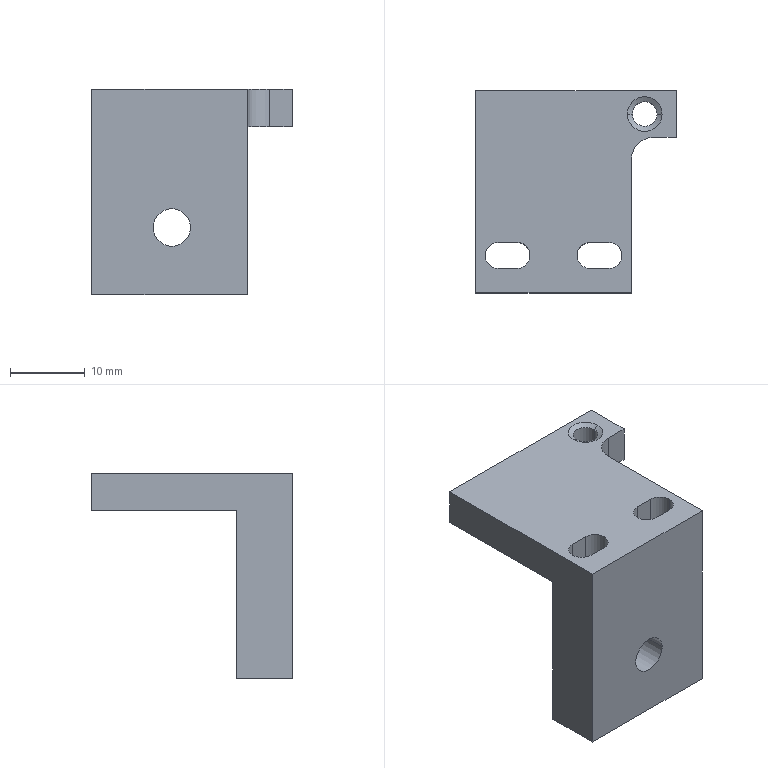Part | NX | 1 solid | 27 faces | box 26.8 x 27 x 27.5 mm | volume 5312 mm3 | plane 14 | cylinder 11 | cone 2 | commonest cylinder face diameters 3.5 x6 3.3 x2 5 x2 6 x1
STEP:
#1=CARTESIAN_POINT('',(6.,-2.5,-13.75));
#2=VERTEX_POINT('',#1);
#3=CARTESIAN_POINT('',(6.,-10.,-13.75));
#4=VERTEX_POINT('',#3);
#5=CARTESIAN_POINT('',(6.,0.,-13.75));
#6=DIRECTION('',(0.,-1.,0.));
#7=VECTOR('',#6,1000.);
#8=LINE('',#5,#7);
#9=EDGE_CURVE('',#2,#4,#8,.T.);
#10=ORIENTED_EDGE('',*,*,#9,.F.);
#11=CARTESIAN_POINT('',(6.,-2.5,8.75));
#12=VERTEX_POINT('',#11);
#13=CARTESIAN_POINT('',(6.,-2.5,0.));
#14=DIRECTION('',(0.,0.,1.));
#15=VECTOR('',#14,1000.);
#16=LINE('',#13,#15);
#17=EDGE_CURVE('',#2,#12,#16,.T.);
#18=ORIENTED_EDGE('',*,*,#17,.T.);
#19=CARTESIAN_POINT('',(6.,7.8,8.75));
#20=VERTEX_POINT('',#19);
#21=CARTESIAN_POINT('',(6.,0.,8.75));
#22=DIRECTION('',(0.,1.,0.));
#23=VECTOR('',#22,1000.);
#24=LINE('',#21,#23);
#25=EDGE_CURVE('',#12,#20,#24,.T.);
#26=ORIENTED_EDGE('',*,*,#25,.T.);
#27=CARTESIAN_POINT('',(6.,7.8,13.75));
#28=VERTEX_POINT('',#27);
#29=CARTESIAN_POINT('',(6.,7.8,0.));
#30=DIRECTION('',(0.,0.,1.));
#31=VECTOR('',#30,1000.);
#32=LINE('',#29,#31);
#33=EDGE_CURVE('',#20,#28,#32,.T.);
#34=ORIENTED_EDGE('',*,*,#33,.T.);
#35=CARTESIAN_POINT('',(6.,-10.,13.75));
#36=VERTEX_POINT('',#35);
#37=CARTESIAN_POINT('',(6.,0.,13.75));
#38=DIRECTION('',(0.,1.,0.));
#39=VECTOR('',#38,1000.);
#40=LINE('',#37,#39);
#41=EDGE_CURVE('',#36,#28,#40,.T.);
#42=ORIENTED_EDGE('',*,*,#41,.F.);
#43=CARTESIAN_POINT('',(6.,-10.,0.));
#44=DIRECTION('',(0.,0.,1.));
#45=VECTOR('',#44,1000.);
#46=LINE('',#43,#45);
#47=EDGE_CURVE('',#4,#36,#46,.T.);
#48=ORIENTED_EDGE('',*,*,#47,.F.);
#49=EDGE_LOOP('',(#10,#18,#26,#34,#42,#48));
#50=FACE_BOUND('',#49,.T.);
#51=CARTESIAN_POINT('',(6.,0.,0.));
#52=DIRECTION('',(-1.,0.,0.));
#53=DIRECTION('',(0.,0.,1.));
#54=AXIS2_PLACEMENT_3D('',#51,#52,#53);
#55=PLANE('',#54);
#56=ADVANCED_FACE('',(#50),#55,.F.);
#57=CARTESIAN_POINT('',(-14.8,-2.5,8.75));
#58=VERTEX_POINT('',#57);
#59=CARTESIAN_POINT('',(0.,-2.5,8.75));
#60=DIRECTION('',(-1.,0.,0.));
#61=VECTOR('',#60,1000.);
#62=LINE('',#59,#61);
#63=EDGE_CURVE('',#12,#58,#62,.T.);
#64=ORIENTED_EDGE('',*,*,#63,.F.);
#65=ORIENTED_EDGE('',*,*,#17,.F.);
#66=CARTESIAN_POINT('',(-14.8,-2.5,-13.75));
#67=VERTEX_POINT('',#66);
#68=CARTESIAN_POINT('',(0.,-2.5,-13.75));
#69=DIRECTION('',(1.,0.,0.));
#70=VECTOR('',#69,1000.);
#71=LINE('',#68,#70);
#72=EDGE_CURVE('',#67,#2,#71,.T.);
#73=ORIENTED_EDGE('',*,*,#72,.F.);
#74=CARTESIAN_POINT('',(-14.8,-2.5,0.));
#75=DIRECTION('',(0.,0.,-1.));
#76=VECTOR('',#75,1000.);
#77=LINE('',#74,#76);
#78=EDGE_CURVE('',#58,#67,#77,.T.);
#79=ORIENTED_EDGE('',*,*,#78,.F.);
#80=EDGE_LOOP('',(#64,#65,#73,#79));
#81=FACE_BOUND('',#80,.T.);
#82=CARTESIAN_POINT('',(-6.6,-2.5,-4.75));
#83=VERTEX_POINT('',#82);
#84=CARTESIAN_POINT('',(-1.6,-2.5,-4.75));
#85=VERTEX_POINT('',#84);
#86=CARTESIAN_POINT('',(-4.1,-2.5,-4.75));
#87=DIRECTION('',(0.,1.,0.));
#88=DIRECTION('',(-1.,0.,0.));
#89=AXIS2_PLACEMENT_3D('',#86,#87,#88);
#90=CIRCLE('',#89,2.5);
#91=EDGE_CURVE('',#83,#85,#90,.T.);
#92=ORIENTED_EDGE('',*,*,#91,.F.);
#93=CARTESIAN_POINT('',(-4.1,-2.5,-4.75));
#94=DIRECTION('',(0.,1.,0.));
#95=DIRECTION('',(-1.,0.,0.));
#96=AXIS2_PLACEMENT_3D('',#93,#94,#95);
#97=CIRCLE('',#96,2.5);
#98=EDGE_CURVE('',#85,#83,#97,.T.);
#99=ORIENTED_EDGE('',*,*,#98,.F.);
#100=EDGE_LOOP('',(#92,#99));
#101=FACE_BOUND('',#100,.T.);
#102=CARTESIAN_POINT('',(0.,-2.5,8.75));
#103=DIRECTION('',(0.,-1.,0.));
#104=DIRECTION('',(0.,0.,-1.));
#105=AXIS2_PLACEMENT_3D('',#102,#103,#104);
#106=PLANE('',#105);
#107=ADVANCED_FACE('',(#81,#101),#106,.F.);
#108=CARTESIAN_POINT('',(9.,10.8,8.75));
#109=VERTEX_POINT('',#108);
#110=CARTESIAN_POINT('',(9.,10.8,13.75));
#111=VERTEX_POINT('',#110);
#112=CARTESIAN_POINT('',(9.,10.8,0.));
#113=DIRECTION('',(0.,0.,1.));
#114=VECTOR('',#113,1000.);
#115=LINE('',#112,#114);
#116=EDGE_CURVE('',#109,#111,#115,.T.);
#117=ORIENTED_EDGE('',*,*,#116,.F.);
#118=CARTESIAN_POINT('',(12.,10.8,8.75));
#119=VERTEX_POINT('',#118);
#120=CARTESIAN_POINT('',(0.,10.8,8.75));
#121=DIRECTION('',(-1.,0.,0.));
#122=VECTOR('',#121,1000.);
#123=LINE('',#120,#122);
#124=EDGE_CURVE('',#119,#109,#123,.T.);
#125=ORIENTED_EDGE('',*,*,#124,.F.);
#126=CARTESIAN_POINT('',(12.,10.8,13.75));
#127=VERTEX_POINT('',#126);
#128=CARTESIAN_POINT('',(12.,10.8,13.75));
#129=DIRECTION('',(0.,0.,-1.));
#130=VECTOR('',#129,1000.);
#131=LINE('',#128,#130);
#132=EDGE_CURVE('',#127,#119,#131,.T.);
#133=ORIENTED_EDGE('',*,*,#132,.F.);
#134=CARTESIAN_POINT('',(0.,10.8,13.75));
#135=DIRECTION('',(-1.,0.,0.));
#136=VECTOR('',#135,1000.);
#137=LINE('',#134,#136);
#138=EDGE_CURVE('',#127,#111,#137,.T.);
#139=ORIENTED_EDGE('',*,*,#138,.T.);
#140=EDGE_LOOP('',(#117,#125,#133,#139));
#141=FACE_BOUND('',#140,.T.);
#142=CARTESIAN_POINT('',(6.,10.8,13.75));
#143=DIRECTION('',(0.,-1.,0.));
#144=DIRECTION('',(0.,0.,-1.));
#145=AXIS2_PLACEMENT_3D('',#142,#143,#144);
#146=PLANE('',#145);
#147=ADVANCED_FACE('',(#141),#146,.T.);
#148=ORIENTED_EDGE('',*,*,#78,.T.);
#149=CARTESIAN_POINT('',(-14.8,-10.,-13.75));
#150=VERTEX_POINT('',#149);
#151=CARTESIAN_POINT('',(-14.8,0.,-13.75));
#152=DIRECTION('',(0.,-1.,0.));
#153=VECTOR('',#152,1000.);
#154=LINE('',#151,#153);
#155=EDGE_CURVE('',#67,#150,#154,.T.);
#156=ORIENTED_EDGE('',*,*,#155,.T.);
#157=CARTESIAN_POINT('',(-14.8,-10.,13.75));
#158=VERTEX_POINT('',#157);
#159=CARTESIAN_POINT('',(-14.8,-10.,0.));
#160=DIRECTION('',(0.,0.,-1.));
#161=VECTOR('',#160,1000.);
#162=LINE('',#159,#161);
#163=EDGE_CURVE('',#158,#150,#162,.T.);
#164=ORIENTED_EDGE('',*,*,#163,.F.);
#165=CARTESIAN_POINT('',(-14.8,17.,13.75));
#166=VERTEX_POINT('',#165);
#167=CARTESIAN_POINT('',(-14.8,0.,13.75));
#168=DIRECTION('',(0.,1.,0.));
#169=VECTOR('',#168,1000.);
#170=LINE('',#167,#169);
#171=EDGE_CURVE('',#158,#166,#170,.T.);
#172=ORIENTED_EDGE('',*,*,#171,.T.);
#173=CARTESIAN_POINT('',(-14.8,17.,8.75));
#174=VERTEX_POINT('',#173);
#175=CARTESIAN_POINT('',(-14.8,17.,0.));
#176=DIRECTION('',(0.,0.,1.));
#177=VECTOR('',#176,1000.);
#178=LINE('',#175,#177);
#179=EDGE_CURVE('',#174,#166,#178,.T.);
#180=ORIENTED_EDGE('',*,*,#179,.F.);
#181=CARTESIAN_POINT('',(-14.8,0.,8.75));
#182=DIRECTION('',(0.,-1.,0.));
#183=VECTOR('',#182,1000.);
#184=LINE('',#181,#183);
#185=EDGE_CURVE('',#174,#58,#184,.T.);
#186=ORIENTED_EDGE('',*,*,#185,.T.);
#187=EDGE_LOOP('',(#148,#156,#164,#172,#180,#186));
#188=FACE_BOUND('',#187,.T.);
#189=CARTESIAN_POINT('',(-14.8,0.,0.));
#190=DIRECTION('',(-1.,0.,0.));
#191=DIRECTION('',(0.,0.,1.));
#192=AXIS2_PLACEMENT_3D('',#189,#190,#191);
#193=PLANE('',#192);
#194=ADVANCED_FACE('',(#188),#193,.T.);
#195=CARTESIAN_POINT('',(12.,17.,13.75));
#196=VERTEX_POINT('',#195);
#197=CARTESIAN_POINT('',(12.,0.,13.75));
#198=DIRECTION('',(0.,-1.,0.));
#199=VECTOR('',#198,1000.);
#200=LINE('',#197,#199);
#201=EDGE_CURVE('',#196,#127,#200,.T.);
#202=ORIENTED_EDGE('',*,*,#201,.T.);
#203=ORIENTED_EDGE('',*,*,#132,.T.);
#204=CARTESIAN_POINT('',(12.,17.,8.75));
#205=VERTEX_POINT('',#204);
#206=CARTESIAN_POINT('',(12.,0.,8.75));
#207=DIRECTION('',(0.,-1.,0.));
#208=VECTOR('',#207,1000.);
#209=LINE('',#206,#208);
#210=EDGE_CURVE('',#205,#119,#209,.T.);
#211=ORIENTED_EDGE('',*,*,#210,.F.);
#212=CARTESIAN_POINT('',(12.,17.,0.));
#213=DIRECTION('',(0.,0.,1.));
#214=VECTOR('',#213,1000.);
#215=LINE('',#212,#214);
#216=EDGE_CURVE('',#205,#196,#215,.T.);
#217=ORIENTED_EDGE('',*,*,#216,.T.);
#218=EDGE_LOOP('',(#202,#203,#211,#217));
#219=FACE_BOUND('',#218,.T.);
#220=CARTESIAN_POINT('',(12.,10.8,13.75));
#221=DIRECTION('',(1.,0.,0.));
#222=DIRECTION('',(0.,1.,0.));
#223=AXIS2_PLACEMENT_3D('',#220,#221,#222);
#224=PLANE('',#223);
#225=ADVANCED_FACE('',(#219),#224,.T.);
#226=CARTESIAN_POINT('',(0.,17.,13.75));
#227=DIRECTION('',(1.,0.,0.));
#228=VECTOR('',#227,1000.);
#229=LINE('',#226,#228);
#230=EDGE_CURVE('',#166,#196,#229,.T.);
#231=ORIENTED_EDGE('',*,*,#230,.T.);
#232=ORIENTED_EDGE('',*,*,#216,.F.);
#233=CARTESIAN_POINT('',(0.,17.,8.75));
#234=DIRECTION('',(1.,0.,0.));
#235=VECTOR('',#234,1000.);
#236=LINE('',#233,#235);
#237=EDGE_CURVE('',#174,#205,#236,.T.);
#238=ORIENTED_EDGE('',*,*,#237,.F.);
#239=ORIENTED_EDGE('',*,*,#179,.T.);
#240=EDGE_LOOP('',(#231,#232,#238,#239));
#241=FACE_BOUND('',#240,.T.);
#242=CARTESIAN_POINT('',(12.,17.,13.75));
#243=DIRECTION('',(0.,1.,0.));
#244=DIRECTION('',(1.,0.,0.));
#245=AXIS2_PLACEMENT_3D('',#242,#243,#244);
#246=PLANE('',#245);
#247=ADVANCED_FACE('',(#241),#246,.T.);
#248=CARTESIAN_POINT('',(0.,-10.,13.75));
#249=DIRECTION('',(-1.,0.,0.));
#250=VECTOR('',#249,1000.);
#251=LINE('',#248,#250);
#252=EDGE_CURVE('',#36,#158,#251,.T.);
#253=ORIENTED_EDGE('',*,*,#252,.T.);
#254=ORIENTED_EDGE('',*,*,#163,.T.);
#255=CARTESIAN_POINT('',(0.,-10.,-13.75));
#256=DIRECTION('',(1.,0.,0.));
#257=VECTOR('',#256,1000.);
#258=LINE('',#255,#257);
#259=EDGE_CURVE('',#150,#4,#258,.T.);
#260=ORIENTED_EDGE('',*,*,#259,.T.);
#261=ORIENTED_EDGE('',*,*,#47,.T.);
#262=EDGE_LOOP('',(#253,#254,#260,#261));
#263=FACE_BOUND('',#262,.T.);
#264=CARTESIAN_POINT('',(-6.6,-10.,-4.75));
#265=VERTEX_POINT('',#264);
#266=CARTESIAN_POINT('',(-1.6,-10.,-4.75));
#267=VERTEX_POINT('',#266);
#268=CARTESIAN_POINT('',(-4.1,-10.,-4.75));
#269=DIRECTION('',(0.,1.,0.));
#270=DIRECTION('',(-1.,0.,0.));
#271=AXIS2_PLACEMENT_3D('',#268,#269,#270);
#272=CIRCLE('',#271,2.5);
#273=EDGE_CURVE('',#265,#267,#272,.T.);
#274=ORIENTED_EDGE('',*,*,#273,.T.);
#275=CARTESIAN_POINT('',(-4.1,-10.,-4.75));
#276=DIRECTION('',(0.,1.,0.));
#277=DIRECTION('',(-1.,0.,0.));
#278=AXIS2_PLACEMENT_3D('',#275,#276,#277);
#279=CIRCLE('',#278,2.5);
#280=EDGE_CURVE('',#267,#265,#279,.T.);
#281=ORIENTED_EDGE('',*,*,#280,.T.);
#282=EDGE_LOOP('',(#274,#281));
#283=FACE_BOUND('',#282,.T.);
#284=CARTESIAN_POINT('',(0.,-10.,-13.75));
#285=DIRECTION('',(0.,-1.,0.));
#286=DIRECTION('',(0.,0.,-1.));
#287=AXIS2_PLACEMENT_3D('',#284,#285,#286);
#288=PLANE('',#287);
#289=ADVANCED_FACE('',(#263,#283),#288,.T.);
#290=ORIENTED_EDGE('',*,*,#9,.T.);
#291=ORIENTED_EDGE('',*,*,#259,.F.);
#292=ORIENTED_EDGE('',*,*,#155,.F.);
#293=ORIENTED_EDGE('',*,*,#72,.T.);
#294=EDGE_LOOP('',(#290,#291,#292,#293));
#295=FACE_BOUND('',#294,.T.);
#296=CARTESIAN_POINT('',(-11.8,-6.75,-13.75));
#297=VERTEX_POINT('',#296);
#298=CARTESIAN_POINT('',(-13.55,-5.,-13.75));
#299=VERTEX_POINT('',#298);
#300=CARTESIAN_POINT('',(-11.8,-5.,-13.75));
#301=DIRECTION('',(0.,0.,-1.));
#302=DIRECTION('',(-1.,0.,0.));
#303=AXIS2_PLACEMENT_3D('',#300,#301,#302);
#304=CIRCLE('',#303,1.75);
#305=EDGE_CURVE('',#297,#299,#304,.T.);
#306=ORIENTED_EDGE('',*,*,#305,.F.);
#307=CARTESIAN_POINT('',(-9.3,-6.75,-13.75));
#308=VERTEX_POINT('',#307);
#309=CARTESIAN_POINT('',(0.,-6.75,-13.75));
#310=DIRECTION('',(1.,0.,0.));
#311=VECTOR('',#310,1000.);
#312=LINE('',#309,#311);
#313=EDGE_CURVE('',#297,#308,#312,.T.);
#314=ORIENTED_EDGE('',*,*,#313,.T.);
#315=CARTESIAN_POINT('',(-9.3,-3.25,-13.75));
#316=VERTEX_POINT('',#315);
#317=CARTESIAN_POINT('',(-9.3,-5.,-13.75));
#318=DIRECTION('',(0.,0.,-1.));
#319=DIRECTION('',(-1.,0.,0.));
#320=AXIS2_PLACEMENT_3D('',#317,#318,#319);
#321=CIRCLE('',#320,1.75);
#322=EDGE_CURVE('',#316,#308,#321,.T.);
#323=ORIENTED_EDGE('',*,*,#322,.F.);
#324=CARTESIAN_POINT('',(-11.8,-3.25,-13.75));
#325=VERTEX_POINT('',#324);
#326=CARTESIAN_POINT('',(0.,-3.25,-13.75));
#327=DIRECTION('',(1.,0.,0.));
#328=VECTOR('',#327,1000.);
#329=LINE('',#326,#328);
#330=EDGE_CURVE('',#325,#316,#329,.T.);
#331=ORIENTED_EDGE('',*,*,#330,.F.);
#332=CARTESIAN_POINT('',(-11.8,-5.,-13.75));
#333=DIRECTION('',(0.,0.,-1.));
#334=DIRECTION('',(-1.,0.,0.));
#335=AXIS2_PLACEMENT_3D('',#332,#333,#334);
#336=CIRCLE('',#335,1.75);
#337=EDGE_CURVE('',#299,#325,#336,.T.);
#338=ORIENTED_EDGE('',*,*,#337,.F.);
#339=EDGE_LOOP('',(#306,#314,#323,#331,#338));
#340=FACE_BOUND('',#339,.T.);
#341=CARTESIAN_POINT('',(3.,-6.75,-13.75));
#342=VERTEX_POINT('',#341);
#343=CARTESIAN_POINT('',(4.75,-5.,-13.75));
#344=VERTEX_POINT('',#343);
#345=CARTESIAN_POINT('',(3.,-5.,-13.75));
#346=DIRECTION('',(0.,0.,1.));
#347=DIRECTION('',(1.,0.,0.));
#348=AXIS2_PLACEMENT_3D('',#345,#346,#347);
#349=CIRCLE('',#348,1.75);
#350=EDGE_CURVE('',#342,#344,#349,.T.);
#351=ORIENTED_EDGE('',*,*,#350,.T.);
#352=CARTESIAN_POINT('',(3.,-3.25,-13.75));
#353=VERTEX_POINT('',#352);
#354=CARTESIAN_POINT('',(3.,-5.,-13.75));
#355=DIRECTION('',(0.,0.,1.));
#356=DIRECTION('',(1.,0.,0.));
#357=AXIS2_PLACEMENT_3D('',#354,#355,#356);
#358=CIRCLE('',#357,1.75);
#359=EDGE_CURVE('',#344,#353,#358,.T.);
#360=ORIENTED_EDGE('',*,*,#359,.T.);
#361=CARTESIAN_POINT('',(0.5,-3.25,-13.75));
#362=VERTEX_POINT('',#361);
#363=CARTESIAN_POINT('',(0.,-3.25,-13.75));
#364=DIRECTION('',(1.,0.,0.));
#365=VECTOR('',#364,1000.);
#366=LINE('',#363,#365);
#367=EDGE_CURVE('',#362,#353,#366,.T.);
#368=ORIENTED_EDGE('',*,*,#367,.F.);
#369=CARTESIAN_POINT('',(0.5,-6.75,-13.75));
#370=VERTEX_POINT('',#369);
#371=CARTESIAN_POINT('',(0.5,-5.,-13.75));
#372=DIRECTION('',(0.,0.,1.));
#373=DIRECTION('',(1.,0.,0.));
#374=AXIS2_PLACEMENT_3D('',#371,#372,#373);
#375=CIRCLE('',#374,1.75);
#376=EDGE_CURVE('',#362,#370,#375,.T.);
#377=ORIENTED_EDGE('',*,*,#376,.T.);
#378=CARTESIAN_POINT('',(0.,-6.75,-13.75));
#379=DIRECTION('',(-1.,0.,0.));
#380=VECTOR('',#379,1000.);
#381=LINE('',#378,#380);
#382=EDGE_CURVE('',#342,#370,#381,.T.);
#383=ORIENTED_EDGE('',*,*,#382,.F.);
#384=EDGE_LOOP('',(#351,#360,#368,#377,#383));
#385=FACE_BOUND('',#384,.T.);
#386=CARTESIAN_POINT('',(0.,17.,-13.75));
#387=DIRECTION('',(0.,0.,-1.));
#388=DIRECTION('',(0.,-1.,0.));
#389=AXIS2_PLACEMENT_3D('',#386,#387,#388);
#390=PLANE('',#389);
#391=ADVANCED_FACE('',(#295,#340,#385),#390,.T.);
#392=ORIENTED_EDGE('',*,*,#230,.F.);
#393=ORIENTED_EDGE('',*,*,#171,.F.);
#394=ORIENTED_EDGE('',*,*,#252,.F.);
#395=ORIENTED_EDGE('',*,*,#41,.T.);
#396=CARTESIAN_POINT('',(9.,7.8,13.75));
#397=DIRECTION('',(0.,0.,1.));
#398=DIRECTION('',(1.,0.,0.));
#399=AXIS2_PLACEMENT_3D('',#396,#397,#398);
#400=CIRCLE('',#399,3.);
#401=EDGE_CURVE('',#111,#28,#400,.T.);
#402=ORIENTED_EDGE('',*,*,#401,.F.);
#403=ORIENTED_EDGE('',*,*,#138,.F.);
#404=ORIENTED_EDGE('',*,*,#201,.F.);
#405=EDGE_LOOP('',(#392,#393,#394,#395,#402,#403,#404));
#406=FACE_BOUND('',#405,.T.);
#407=CARTESIAN_POINT('',(-9.3,-3.25,13.75));
#408=VERTEX_POINT('',#407);
#409=CARTESIAN_POINT('',(-9.3,-6.75,13.75));
#410=VERTEX_POINT('',#409);
#411=CARTESIAN_POINT('',(-9.3,-5.,13.75));
#412=DIRECTION('',(0.,0.,-1.));
#413=DIRECTION('',(-1.,0.,0.));
#414=AXIS2_PLACEMENT_3D('',#411,#412,#413);
#415=CIRCLE('',#414,1.75);
#416=EDGE_CURVE('',#408,#410,#415,.T.);
#417=ORIENTED_EDGE('',*,*,#416,.T.);
#418=CARTESIAN_POINT('',(-11.8,-6.75,13.75));
#419=VERTEX_POINT('',#418);
#420=CARTESIAN_POINT('',(0.,-6.75,13.75));
#421=DIRECTION('',(-1.,0.,0.));
#422=VECTOR('',#421,1000.);
#423=LINE('',#420,#422);
#424=EDGE_CURVE('',#410,#419,#423,.T.);
#425=ORIENTED_EDGE('',*,*,#424,.T.);
#426=CARTESIAN_POINT('',(-13.55,-5.,13.75));
#427=VERTEX_POINT('',#426);
#428=CARTESIAN_POINT('',(-11.8,-5.,13.75));
#429=DIRECTION('',(0.,0.,-1.));
#430=DIRECTION('',(-1.,0.,0.));
#431=AXIS2_PLACEMENT_3D('',#428,#429,#430);
#432=CIRCLE('',#431,1.75);
#433=EDGE_CURVE('',#419,#427,#432,.T.);
#434=ORIENTED_EDGE('',*,*,#433,.T.);
#435=CARTESIAN_POINT('',(-11.8,-3.25,13.75));
#436=VERTEX_POINT('',#435);
#437=CARTESIAN_POINT('',(-11.8,-5.,13.75));
#438=DIRECTION('',(0.,0.,-1.));
#439=DIRECTION('',(-1.,0.,0.));
#440=AXIS2_PLACEMENT_3D('',#437,#438,#439);
#441=CIRCLE('',#440,1.75);
#442=EDGE_CURVE('',#427,#436,#441,.T.);
#443=ORIENTED_EDGE('',*,*,#442,.T.);
#444=CARTESIAN_POINT('',(0.,-3.25,13.75));
#445=DIRECTION('',(1.,0.,0.));
#446=VECTOR('',#445,1000.);
#447=LINE('',#444,#446);
#448=EDGE_CURVE('',#436,#408,#447,.T.);
#449=ORIENTED_EDGE('',*,*,#448,.T.);
#450=EDGE_LOOP('',(#417,#425,#434,#443,#449));
#451=FACE_BOUND('',#450,.T.);
#452=CARTESIAN_POINT('',(10.115,13.9,13.75));
#453=VERTEX_POINT('',#452);
#454=CARTESIAN_POINT('',(5.485,13.9,13.75));
#455=VERTEX_POINT('',#454);
#456=CARTESIAN_POINT('',(7.8,13.9,13.75));
#457=DIRECTION('',(0.,0.,1.));
#458=DIRECTION('',(1.,0.,0.));
#459=AXIS2_PLACEMENT_3D('',#456,#457,#458);
#460=CIRCLE('',#459,2.315);
#461=EDGE_CURVE('',#453,#455,#460,.T.);
#462=ORIENTED_EDGE('',*,*,#461,.F.);
#463=CARTESIAN_POINT('',(7.8,13.9,13.75));
#464=DIRECTION('',(0.,0.,1.));
#465=DIRECTION('',(1.,0.,0.));
#466=AXIS2_PLACEMENT_3D('',#463,#464,#465);
#467=CIRCLE('',#466,2.315);
#468=EDGE_CURVE('',#455,#453,#467,.T.);
#469=ORIENTED_EDGE('',*,*,#468,.F.);
#470=EDGE_LOOP('',(#462,#469));
#471=FACE_BOUND('',#470,.T.);
#472=CARTESIAN_POINT('',(3.,-6.75,13.75));
#473=VERTEX_POINT('',#472);
#474=CARTESIAN_POINT('',(4.75,-5.,13.75));
#475=VERTEX_POINT('',#474);
#476=CARTESIAN_POINT('',(3.,-5.,13.75));
#477=DIRECTION('',(0.,0.,1.));
#478=DIRECTION('',(1.,0.,0.));
#479=AXIS2_PLACEMENT_3D('',#476,#477,#478);
#480=CIRCLE('',#479,1.75);
#481=EDGE_CURVE('',#473,#475,#480,.T.);
#482=ORIENTED_EDGE('',*,*,#481,.F.);
#483=CARTESIAN_POINT('',(0.5,-6.75,13.75));
#484=VERTEX_POINT('',#483);
#485=CARTESIAN_POINT('',(0.,-6.75,13.75));
#486=DIRECTION('',(1.,0.,0.));
#487=VECTOR('',#486,1000.);
#488=LINE('',#485,#487);
#489=EDGE_CURVE('',#484,#473,#488,.T.);
#490=ORIENTED_EDGE('',*,*,#489,.F.);
#491=CARTESIAN_POINT('',(0.5,-3.25,13.75));
#492=VERTEX_POINT('',#491);
#493=CARTESIAN_POINT('',(0.5,-5.,13.75));
#494=DIRECTION('',(0.,0.,1.));
#495=DIRECTION('',(1.,0.,0.));
#496=AXIS2_PLACEMENT_3D('',#493,#494,#495);
#497=CIRCLE('',#496,1.75);
#498=EDGE_CURVE('',#492,#484,#497,.T.);
#499=ORIENTED_EDGE('',*,*,#498,.F.);
#500=CARTESIAN_POINT('',(3.,-3.25,13.75));
#501=VERTEX_POINT('',#500);
#502=CARTESIAN_POINT('',(0.,-3.25,13.75));
#503=DIRECTION('',(-1.,0.,0.));
#504=VECTOR('',#503,1000.);
#505=LINE('',#502,#504);
#506=EDGE_CURVE('',#501,#492,#505,.T.);
#507=ORIENTED_EDGE('',*,*,#506,.F.);
#508=CARTESIAN_POINT('',(3.,-5.,13.75));
#509=DIRECTION('',(0.,0.,1.));
#510=DIRECTION('',(1.,0.,0.));
#511=AXIS2_PLACEMENT_3D('',#508,#509,#510);
#512=CIRCLE('',#511,1.75);
#513=EDGE_CURVE('',#475,#501,#512,.T.);
#514=ORIENTED_EDGE('',*,*,#513,.F.);
#515=EDGE_LOOP('',(#482,#490,#499,#507,#514));
#516=FACE_BOUND('',#515,.T.);
#517=CARTESIAN_POINT('',(0.,-10.,13.75));
#518=DIRECTION('',(0.,0.,1.));
#519=DIRECTION('',(1.,0.,0.));
#520=AXIS2_PLACEMENT_3D('',#517,#518,#519);
#521=PLANE('',#520);
#522=ADVANCED_FACE('',(#406,#451,#471,#516),#521,.T.);
#523=CARTESIAN_POINT('',(6.15,13.9,8.75));
#524=VERTEX_POINT('',#523);
#525=CARTESIAN_POINT('',(9.45,13.9,8.75));
#526=VERTEX_POINT('',#525);
#527=CARTESIAN_POINT('',(7.8,13.9,8.75));
#528=DIRECTION('',(0.,0.,-1.));
#529=DIRECTION('',(-1.,0.,0.));
#530=AXIS2_PLACEMENT_3D('',#527,#528,#529);
#531=CIRCLE('',#530,1.65);
#532=EDGE_CURVE('',#524,#526,#531,.T.);
#533=ORIENTED_EDGE('',*,*,#532,.T.);
#534=CARTESIAN_POINT('',(9.45,13.9,13.366));
#535=VERTEX_POINT('',#534);
#536=CARTESIAN_POINT('',(9.45,13.9,11.25));
#537=DIRECTION('',(0.,0.,1.));
#538=VECTOR('',#537,1000.);
#539=LINE('',#536,#538);
#540=EDGE_CURVE('',#526,#535,#539,.T.);
#541=ORIENTED_EDGE('',*,*,#540,.T.);
#542=CARTESIAN_POINT('',(6.15,13.9,13.366));
#543=VERTEX_POINT('',#542);
#544=CARTESIAN_POINT('',(7.8,13.9,13.366));
#545=DIRECTION('',(0.,0.,1.));
#546=DIRECTION('',(1.,0.,0.));
#547=AXIS2_PLACEMENT_3D('',#544,#545,#546);
#548=CIRCLE('',#547,1.65);
#549=EDGE_CURVE('',#535,#543,#548,.T.);
#550=ORIENTED_EDGE('',*,*,#549,.T.);
#551=CARTESIAN_POINT('',(6.15,13.9,11.25));
#552=DIRECTION('',(0.,0.,1.));
#553=VECTOR('',#552,1000.);
#554=LINE('',#551,#553);
#555=EDGE_CURVE('',#524,#543,#554,.T.);
#556=ORIENTED_EDGE('',*,*,#555,.F.);
#557=EDGE_LOOP('',(#533,#541,#550,#556));
#558=FACE_BOUND('',#557,.T.);
#559=CARTESIAN_POINT('',(7.8,13.9,11.25));
#560=DIRECTION('',(0.,0.,1.));
#561=DIRECTION('',(-1.,0.,0.));
#562=AXIS2_PLACEMENT_3D('',#559,#560,#561);
#563=CYLINDRICAL_SURFACE('',#562,1.65);
#564=ADVANCED_FACE('',(#558),#563,.F.);
#565=ORIENTED_EDGE('',*,*,#91,.T.);
#566=CARTESIAN_POINT('',(-1.6,-10.,-4.75));
#567=DIRECTION('',(0.,-1.,0.));
#568=VECTOR('',#567,1000.);
#569=LINE('',#566,#568);
#570=EDGE_CURVE('',#267,#85,#569,.F.);
#571=ORIENTED_EDGE('',*,*,#570,.F.);
#572=ORIENTED_EDGE('',*,*,#273,.F.);
#573=CARTESIAN_POINT('',(-6.6,-10.,-4.75));
#574=DIRECTION('',(0.,-1.,0.));
#575=VECTOR('',#574,1000.);
#576=LINE('',#573,#575);
#577=EDGE_CURVE('',#265,#83,#576,.F.);
#578=ORIENTED_EDGE('',*,*,#577,.T.);
#579=EDGE_LOOP('',(#565,#571,#572,#578));
#580=FACE_BOUND('',#579,.T.);
#581=CARTESIAN_POINT('',(-4.1,-10.,-4.75));
#582=DIRECTION('',(0.,-1.,0.));
#583=DIRECTION('',(-1.,0.,0.));
#584=AXIS2_PLACEMENT_3D('',#581,#582,#583);
#585=CYLINDRICAL_SURFACE('',#584,2.5);
#586=ADVANCED_FACE('',(#580),#585,.F.);
#587=CARTESIAN_POINT('',(-9.3,-3.25,-16.5));
#588=DIRECTION('',(0.,0.,1.));
#589=VECTOR('',#588,1000.);
#590=LINE('',#587,#589);
#591=EDGE_CURVE('',#316,#408,#590,.T.);
#592=ORIENTED_EDGE('',*,*,#591,.T.);
#593=ORIENTED_EDGE('',*,*,#448,.F.);
#594=CARTESIAN_POINT('',(-11.8,-3.25,-16.5));
#595=DIRECTION('',(0.,0.,1.));
#596=VECTOR('',#595,1000.);
#597=LINE('',#594,#596);
#598=EDGE_CURVE('',#325,#436,#597,.T.);
#599=ORIENTED_EDGE('',*,*,#598,.F.);
#600=ORIENTED_EDGE('',*,*,#330,.T.);
#601=EDGE_LOOP('',(#592,#593,#599,#600));
#602=FACE_BOUND('',#601,.T.);
#603=CARTESIAN_POINT('',(-8.8,-3.25,-16.5));
#604=DIRECTION('',(0.,-1.,0.));
#605=DIRECTION('',(0.,0.,-1.));
#606=AXIS2_PLACEMENT_3D('',#603,#604,#605);
#607=PLANE('',#606);
#608=ADVANCED_FACE('',(#602),#607,.T.);
#609=CARTESIAN_POINT('',(-13.55,-5.,-16.5));
#610=DIRECTION('',(0.,0.,1.));
#611=VECTOR('',#610,1000.);
#612=LINE('',#609,#611);
#613=EDGE_CURVE('',#299,#427,#612,.T.);
#614=ORIENTED_EDGE('',*,*,#613,.F.);
#615=ORIENTED_EDGE('',*,*,#337,.T.);
#616=ORIENTED_EDGE('',*,*,#598,.T.);
#617=ORIENTED_EDGE('',*,*,#442,.F.);
#618=EDGE_LOOP('',(#614,#615,#616,#617));
#619=FACE_BOUND('',#618,.T.);
#620=CARTESIAN_POINT('',(-11.8,-5.,-16.5));
#621=DIRECTION('',(0.,0.,1.));
#622=DIRECTION('',(-1.,0.,0.));
#623=AXIS2_PLACEMENT_3D('',#620,#621,#622);
#624=CYLINDRICAL_SURFACE('',#623,1.75);
#625=ADVANCED_FACE('',(#619),#624,.F.);
#626=CARTESIAN_POINT('',(-9.3,-6.75,-16.5));
#627=DIRECTION('',(0.,0.,1.));
#628=VECTOR('',#627,1000.);
#629=LINE('',#626,#628);
#630=EDGE_CURVE('',#308,#410,#629,.T.);
#631=ORIENTED_EDGE('',*,*,#630,.T.);
#632=ORIENTED_EDGE('',*,*,#416,.F.);
#633=ORIENTED_EDGE('',*,*,#591,.F.);
#634=ORIENTED_EDGE('',*,*,#322,.T.);
#635=EDGE_LOOP('',(#631,#632,#633,#634));
#636=FACE_BOUND('',#635,.T.);
#637=CARTESIAN_POINT('',(-9.3,-5.,-16.5));
#638=DIRECTION('',(0.,0.,1.));
#639=DIRECTION('',(-1.,0.,0.));
#640=AXIS2_PLACEMENT_3D('',#637,#638,#639);
#641=CYLINDRICAL_SURFACE('',#640,1.75);
#642=ADVANCED_FACE('',(#636),#641,.F.);
#643=CARTESIAN_POINT('',(-11.8,-6.75,-16.5));
#644=DIRECTION('',(0.,0.,1.));
#645=VECTOR('',#644,1000.);
#646=LINE('',#643,#645);
#647=EDGE_CURVE('',#297,#419,#646,.T.);
#648=ORIENTED_EDGE('',*,*,#647,.T.);
#649=ORIENTED_EDGE('',*,*,#424,.F.);
#650=ORIENTED_EDGE('',*,*,#630,.F.);
#651=ORIENTED_EDGE('',*,*,#313,.F.);
#652=EDGE_LOOP('',(#648,#649,#650,#651));
#653=FACE_BOUND('',#652,.T.);
#654=CARTESIAN_POINT('',(-17.,-6.75,-16.5));
#655=DIRECTION('',(0.,1.,0.));
#656=DIRECTION('',(1.,0.,0.));
#657=AXIS2_PLACEMENT_3D('',#654,#655,#656);
#658=PLANE('',#657);
#659=ADVANCED_FACE('',(#653),#658,.T.);
#660=ORIENTED_EDGE('',*,*,#210,.T.);
#661=ORIENTED_EDGE('',*,*,#124,.T.);
#662=CARTESIAN_POINT('',(9.,7.8,8.75));
#663=DIRECTION('',(0.,0.,1.));
#664=DIRECTION('',(1.,0.,0.));
#665=AXIS2_PLACEMENT_3D('',#662,#663,#664);
#666=CIRCLE('',#665,3.);
#667=EDGE_CURVE('',#109,#20,#666,.T.);
#668=ORIENTED_EDGE('',*,*,#667,.T.);
#669=ORIENTED_EDGE('',*,*,#25,.F.);
#670=ORIENTED_EDGE('',*,*,#63,.T.);
#671=ORIENTED_EDGE('',*,*,#185,.F.);
#672=ORIENTED_EDGE('',*,*,#237,.T.);
#673=EDGE_LOOP('',(#660,#661,#668,#669,#670,#671,#672));
#674=FACE_BOUND('',#673,.T.);
#675=ORIENTED_EDGE('',*,*,#532,.F.);
#676=CARTESIAN_POINT('',(7.8,13.9,8.75));
#677=DIRECTION('',(0.,0.,-1.));
#678=DIRECTION('',(-1.,0.,0.));
#679=AXIS2_PLACEMENT_3D('',#676,#677,#678);
#680=CIRCLE('',#679,1.65);
#681=EDGE_CURVE('',#526,#524,#680,.T.);
#682=ORIENTED_EDGE('',*,*,#681,.F.);
#683=EDGE_LOOP('',(#675,#682));
#684=FACE_BOUND('',#683,.T.);
#685=CARTESIAN_POINT('',(-1.172,6.157,8.75));
#686=DIRECTION('',(0.,0.,1.));
#687=DIRECTION('',(1.,0.,0.));
#688=AXIS2_PLACEMENT_3D('',#685,#686,#687);
#689=PLANE('',#688);
#690=ADVANCED_FACE('',(#674,#684),#689,.F.);
#691=ORIENTED_EDGE('',*,*,#461,.T.);
#692=CARTESIAN_POINT('',(6.15,13.9,13.366));
#693=DIRECTION('',(-0.866,0.,0.5));
#694=VECTOR('',#693,1000.);
#695=LINE('',#692,#694);
#696=EDGE_CURVE('',#455,#543,#695,.F.);
#697=ORIENTED_EDGE('',*,*,#696,.T.);
#698=ORIENTED_EDGE('',*,*,#549,.F.);
#699=CARTESIAN_POINT('',(9.45,13.9,13.366));
#700=DIRECTION('',(0.866,0.,0.5));
#701=VECTOR('',#700,1000.);
#702=LINE('',#699,#701);
#703=EDGE_CURVE('',#453,#535,#702,.F.);
#704=ORIENTED_EDGE('',*,*,#703,.F.);
#705=EDGE_LOOP('',(#691,#697,#698,#704));
#706=FACE_BOUND('',#705,.T.);
#707=CARTESIAN_POINT('',(7.8,13.9,13.366));
#708=DIRECTION('',(0.,0.,1.));
#709=DIRECTION('',(1.,0.,0.));
#710=AXIS2_PLACEMENT_3D('',#707,#708,#709);
#711=CONICAL_SURFACE('',#710,1.65,1.047);
#712=ADVANCED_FACE('',(#706),#711,.F.);
#713=ORIENTED_EDGE('',*,*,#116,.T.);
#714=ORIENTED_EDGE('',*,*,#401,.T.);
#715=ORIENTED_EDGE('',*,*,#33,.F.);
#716=ORIENTED_EDGE('',*,*,#667,.F.);
#717=EDGE_LOOP('',(#713,#714,#715,#716));
#718=FACE_BOUND('',#717,.T.);
#719=CARTESIAN_POINT('',(9.,7.8,0.));
#720=DIRECTION('',(0.,0.,1.));
#721=DIRECTION('',(1.,0.,0.));
#722=AXIS2_PLACEMENT_3D('',#719,#720,#721);
#723=CYLINDRICAL_SURFACE('',#722,3.);
#724=ADVANCED_FACE('',(#718),#723,.F.);
#725=CARTESIAN_POINT('',(4.75,-5.,-16.5));
#726=DIRECTION('',(0.,0.,1.));
#727=VECTOR('',#726,1000.);
#728=LINE('',#725,#727);
#729=EDGE_CURVE('',#344,#475,#728,.T.);
#730=ORIENTED_EDGE('',*,*,#729,.F.);
#731=ORIENTED_EDGE('',*,*,#350,.F.);
#732=CARTESIAN_POINT('',(3.,-6.75,-16.5));
#733=DIRECTION('',(0.,0.,1.));
#734=VECTOR('',#733,1000.);
#735=LINE('',#732,#734);
#736=EDGE_CURVE('',#342,#473,#735,.T.);
#737=ORIENTED_EDGE('',*,*,#736,.T.);
#738=ORIENTED_EDGE('',*,*,#481,.T.);
#739=EDGE_LOOP('',(#730,#731,#737,#738));
#740=FACE_BOUND('',#739,.T.);
#741=CARTESIAN_POINT('',(3.,-5.,-16.5));
#742=DIRECTION('',(0.,0.,1.));
#743=DIRECTION('',(1.,0.,0.));
#744=AXIS2_PLACEMENT_3D('',#741,#742,#743);
#745=CYLINDRICAL_SURFACE('',#744,1.75);
#746=ADVANCED_FACE('',(#740),#745,.F.);
#747=ORIENTED_EDGE('',*,*,#489,.T.);
#748=ORIENTED_EDGE('',*,*,#736,.F.);
#749=ORIENTED_EDGE('',*,*,#382,.T.);
#750=CARTESIAN_POINT('',(0.5,-6.75,-16.5));
#751=DIRECTION('',(0.,0.,1.));
#752=VECTOR('',#751,1000.);
#753=LINE('',#750,#752);
#754=EDGE_CURVE('',#370,#484,#753,.T.);
#755=ORIENTED_EDGE('',*,*,#754,.T.);
#756=EDGE_LOOP('',(#747,#748,#749,#755));
#757=FACE_BOUND('',#756,.T.);
#758=CARTESIAN_POINT('',(3.,-6.75,-16.5));
#759=DIRECTION('',(0.,-1.,0.));
#760=DIRECTION('',(0.,0.,-1.));
#761=AXIS2_PLACEMENT_3D('',#758,#759,#760);
#762=PLANE('',#761);
#763=ADVANCED_FACE('',(#757),#762,.F.);
#764=ORIENTED_EDGE('',*,*,#376,.F.);
#765=CARTESIAN_POINT('',(0.5,-3.25,-16.5));
#766=DIRECTION('',(0.,0.,1.));
#767=VECTOR('',#766,1000.);
#768=LINE('',#765,#767);
#769=EDGE_CURVE('',#362,#492,#768,.T.);
#770=ORIENTED_EDGE('',*,*,#769,.T.);
#771=ORIENTED_EDGE('',*,*,#498,.T.);
#772=ORIENTED_EDGE('',*,*,#754,.F.);
#773=EDGE_LOOP('',(#764,#770,#771,#772));
#774=FACE_BOUND('',#773,.T.);
#775=CARTESIAN_POINT('',(0.5,-5.,-16.5));
#776=DIRECTION('',(0.,0.,1.));
#777=DIRECTION('',(1.,0.,0.));
#778=AXIS2_PLACEMENT_3D('',#775,#776,#777);
#779=CYLINDRICAL_SURFACE('',#778,1.75);
#780=ADVANCED_FACE('',(#774),#779,.F.);
#781=ORIENTED_EDGE('',*,*,#367,.T.);
#782=CARTESIAN_POINT('',(3.,-3.25,-16.5));
#783=DIRECTION('',(0.,0.,1.));
#784=VECTOR('',#783,1000.);
#785=LINE('',#782,#784);
#786=EDGE_CURVE('',#353,#501,#785,.T.);
#787=ORIENTED_EDGE('',*,*,#786,.T.);
#788=ORIENTED_EDGE('',*,*,#506,.T.);
#789=ORIENTED_EDGE('',*,*,#769,.F.);
#790=EDGE_LOOP('',(#781,#787,#788,#789));
#791=FACE_BOUND('',#790,.T.);
#792=CARTESIAN_POINT('',(0.5,-3.25,-16.5));
#793=DIRECTION('',(0.,1.,0.));
#794=DIRECTION('',(1.,0.,0.));
#795=AXIS2_PLACEMENT_3D('',#792,#793,#794);
#796=PLANE('',#795);
#797=ADVANCED_FACE('',(#791),#796,.F.);
#798=ORIENTED_EDGE('',*,*,#577,.F.);
#799=ORIENTED_EDGE('',*,*,#280,.F.);
#800=ORIENTED_EDGE('',*,*,#570,.T.);
#801=ORIENTED_EDGE('',*,*,#98,.T.);
#802=EDGE_LOOP('',(#798,#799,#800,#801));
#803=FACE_BOUND('',#802,.T.);
#804=CARTESIAN_POINT('',(-4.1,-10.,-4.75));
#805=DIRECTION('',(0.,-1.,0.));
#806=DIRECTION('',(-1.,0.,0.));
#807=AXIS2_PLACEMENT_3D('',#804,#805,#806);
#808=CYLINDRICAL_SURFACE('',#807,2.5);
#809=ADVANCED_FACE('',(#803),#808,.F.);
#810=CARTESIAN_POINT('',(7.8,13.9,13.366));
#811=DIRECTION('',(0.,0.,1.));
#812=DIRECTION('',(1.,0.,0.));
#813=AXIS2_PLACEMENT_3D('',#810,#811,#812);
#814=CIRCLE('',#813,1.65);
#815=EDGE_CURVE('',#543,#535,#814,.T.);
#816=ORIENTED_EDGE('',*,*,#815,.F.);
#817=ORIENTED_EDGE('',*,*,#696,.F.);
#818=ORIENTED_EDGE('',*,*,#468,.T.);
#819=ORIENTED_EDGE('',*,*,#703,.T.);
#820=EDGE_LOOP('',(#816,#817,#818,#819));
#821=FACE_BOUND('',#820,.T.);
#822=CARTESIAN_POINT('',(7.8,13.9,13.366));
#823=DIRECTION('',(0.,0.,1.));
#824=DIRECTION('',(1.,0.,0.));
#825=AXIS2_PLACEMENT_3D('',#822,#823,#824);
#826=CONICAL_SURFACE('',#825,1.65,1.047);
#827=ADVANCED_FACE('',(#821),#826,.F.);
#828=ORIENTED_EDGE('',*,*,#815,.T.);
#829=ORIENTED_EDGE('',*,*,#540,.F.);
#830=ORIENTED_EDGE('',*,*,#681,.T.);
#831=ORIENTED_EDGE('',*,*,#555,.T.);
#832=EDGE_LOOP('',(#828,#829,#830,#831));
#833=FACE_BOUND('',#832,.T.);
#834=CARTESIAN_POINT('',(7.8,13.9,11.25));
#835=DIRECTION('',(0.,0.,1.));
#836=DIRECTION('',(-1.,0.,0.));
#837=AXIS2_PLACEMENT_3D('',#834,#835,#836);
#838=CYLINDRICAL_SURFACE('',#837,1.65);
#839=ADVANCED_FACE('',(#833),#838,.F.);
#840=ORIENTED_EDGE('',*,*,#359,.F.);
#841=ORIENTED_EDGE('',*,*,#729,.T.);
#842=ORIENTED_EDGE('',*,*,#513,.T.);
#843=ORIENTED_EDGE('',*,*,#786,.F.);
#844=EDGE_LOOP('',(#840,#841,#842,#843));
#845=FACE_BOUND('',#844,.T.);
#846=CARTESIAN_POINT('',(3.,-5.,-16.5));
#847=DIRECTION('',(0.,0.,1.));
#848=DIRECTION('',(1.,0.,0.));
#849=AXIS2_PLACEMENT_3D('',#846,#847,#848);
#850=CYLINDRICAL_SURFACE('',#849,1.75);
#851=ADVANCED_FACE('',(#845),#850,.F.);
#852=ORIENTED_EDGE('',*,*,#305,.T.);
#853=ORIENTED_EDGE('',*,*,#613,.T.);
#854=ORIENTED_EDGE('',*,*,#433,.F.);
#855=ORIENTED_EDGE('',*,*,#647,.F.);
#856=EDGE_LOOP('',(#852,#853,#854,#855));
#857=FACE_BOUND('',#856,.T.);
#858=CARTESIAN_POINT('',(-11.8,-5.,-16.5));
#859=DIRECTION('',(0.,0.,1.));
#860=DIRECTION('',(-1.,0.,0.));
#861=AXIS2_PLACEMENT_3D('',#858,#859,#860);
#862=CYLINDRICAL_SURFACE('',#861,1.75);
#863=ADVANCED_FACE('',(#857),#862,.F.);
#864=CLOSED_SHELL('',(#56,#107,#147,#194,#225,#247,#289,#391,#522,#564,#586,#608,#625,#642,#659,#690,#712,#724,#746,#763,#780,#797,#809,#827,#839,#851,#863));
#865=MANIFOLD_SOLID_BREP('',#864);
#866=(LENGTH_UNIT()NAMED_UNIT(*)SI_UNIT(.MILLI.,.METRE.));
#867=UNCERTAINTY_MEASURE_WITH_UNIT(LENGTH_MEASURE(0.00001),#866,'','');
#868=(NAMED_UNIT(*)PLANE_ANGLE_UNIT()SI_UNIT($,.RADIAN.));
#869=(NAMED_UNIT(*)SI_UNIT($,.STERADIAN.)SOLID_ANGLE_UNIT());
#870=(GEOMETRIC_REPRESENTATION_CONTEXT(3)GLOBAL_UNCERTAINTY_ASSIGNED_CONTEXT((#867))GLOBAL_UNIT_ASSIGNED_CONTEXT((#866,#868,#869))REPRESENTATION_CONTEXT('',''));
#871=ADVANCED_BREP_SHAPE_REPRESENTATION('',(#865),#870);